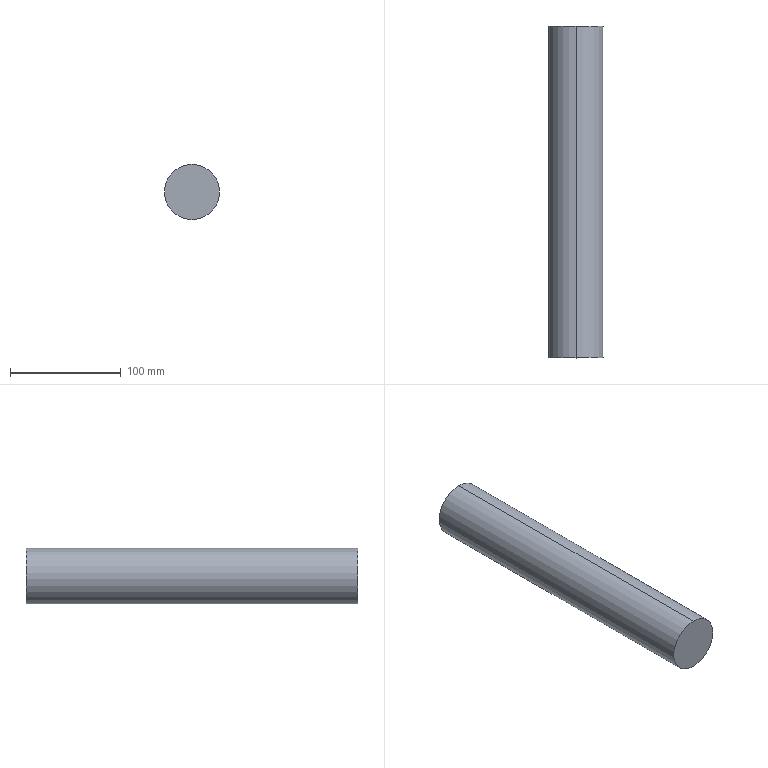Part | STEP file | Tie rod 2 | 1 solid | 4 faces | box 50 x 300 x 50 mm | volume 589049 mm3 | cylinder 2 | plane 2 | commonest cylinder face diameters 50 x2
STEP:
#1=CARTESIAN_POINT('',(0.,300.,25.));
#2=VERTEX_POINT('',#1);
#3=CARTESIAN_POINT('',(0.,300.,-25.));
#4=VERTEX_POINT('',#3);
#5=CARTESIAN_POINT('',(0.,300.,0.));
#6=DIRECTION('',(0.,1.,0.));
#7=DIRECTION('',(0.,0.,1.));
#8=AXIS2_PLACEMENT_3D('',#5,#6,#7);
#9=CIRCLE('',#8,25.);
#10=EDGE_CURVE('',#2,#4,#9,.T.);
#11=ORIENTED_EDGE('',*,*,#10,.F.);
#12=CARTESIAN_POINT('',(0.,0.,25.));
#13=VERTEX_POINT('',#12);
#14=CARTESIAN_POINT('',(0.,300.,25.));
#15=DIRECTION('',(0.,-1.,0.));
#16=VECTOR('',#15,1000.);
#17=LINE('',#14,#16);
#18=EDGE_CURVE('',#2,#13,#17,.T.);
#19=ORIENTED_EDGE('',*,*,#18,.T.);
#20=CARTESIAN_POINT('',(0.,0.,-25.));
#21=VERTEX_POINT('',#20);
#22=CARTESIAN_POINT('',(0.,0.,0.));
#23=DIRECTION('',(0.,1.,0.));
#24=DIRECTION('',(0.,0.,1.));
#25=AXIS2_PLACEMENT_3D('',#22,#23,#24);
#26=CIRCLE('',#25,25.);
#27=EDGE_CURVE('',#13,#21,#26,.T.);
#28=ORIENTED_EDGE('',*,*,#27,.T.);
#29=CARTESIAN_POINT('',(0.,300.,-25.));
#30=DIRECTION('',(0.,-1.,0.));
#31=VECTOR('',#30,1000.);
#32=LINE('',#29,#31);
#33=EDGE_CURVE('',#4,#21,#32,.T.);
#34=ORIENTED_EDGE('',*,*,#33,.F.);
#35=EDGE_LOOP('',(#11,#19,#28,#34));
#36=FACE_OUTER_BOUND('',#35,.T.);
#37=CARTESIAN_POINT('',(0.,300.,0.));
#38=DIRECTION('',(0.,-1.,0.));
#39=DIRECTION('',(0.,0.,-1.));
#40=AXIS2_PLACEMENT_3D('',#37,#38,#39);
#41=CYLINDRICAL_SURFACE('',#40,25.);
#42=ADVANCED_FACE('',(#36),#41,.T.);
#43=ORIENTED_EDGE('',*,*,#18,.F.);
#44=CARTESIAN_POINT('',(0.,300.,0.));
#45=DIRECTION('',(0.,1.,0.));
#46=DIRECTION('',(0.,0.,1.));
#47=AXIS2_PLACEMENT_3D('',#44,#45,#46);
#48=CIRCLE('',#47,25.);
#49=EDGE_CURVE('',#4,#2,#48,.T.);
#50=ORIENTED_EDGE('',*,*,#49,.F.);
#51=ORIENTED_EDGE('',*,*,#33,.T.);
#52=CARTESIAN_POINT('',(0.,0.,0.));
#53=DIRECTION('',(0.,1.,0.));
#54=DIRECTION('',(0.,0.,1.));
#55=AXIS2_PLACEMENT_3D('',#52,#53,#54);
#56=CIRCLE('',#55,25.);
#57=EDGE_CURVE('',#21,#13,#56,.T.);
#58=ORIENTED_EDGE('',*,*,#57,.T.);
#59=EDGE_LOOP('',(#43,#50,#51,#58));
#60=FACE_OUTER_BOUND('',#59,.T.);
#61=CARTESIAN_POINT('',(0.,300.,0.));
#62=DIRECTION('',(0.,-1.,0.));
#63=DIRECTION('',(0.,0.,-1.));
#64=AXIS2_PLACEMENT_3D('',#61,#62,#63);
#65=CYLINDRICAL_SURFACE('',#64,25.);
#66=ADVANCED_FACE('',(#60),#65,.T.);
#67=ORIENTED_EDGE('',*,*,#49,.T.);
#68=ORIENTED_EDGE('',*,*,#10,.T.);
#69=EDGE_LOOP('',(#67,#68));
#70=FACE_OUTER_BOUND('',#69,.T.);
#71=CARTESIAN_POINT('',(0.,300.,0.));
#72=DIRECTION('',(0.,1.,0.));
#73=DIRECTION('',(0.,0.,1.));
#74=AXIS2_PLACEMENT_3D('',#71,#72,#73);
#75=PLANE('',#74);
#76=ADVANCED_FACE('',(#70),#75,.T.);
#77=ORIENTED_EDGE('',*,*,#57,.F.);
#78=ORIENTED_EDGE('',*,*,#27,.F.);
#79=EDGE_LOOP('',(#77,#78));
#80=FACE_OUTER_BOUND('',#79,.T.);
#81=CARTESIAN_POINT('',(0.,0.,0.));
#82=DIRECTION('',(0.,1.,0.));
#83=DIRECTION('',(0.,0.,1.));
#84=AXIS2_PLACEMENT_3D('',#81,#82,#83);
#85=PLANE('',#84);
#86=ADVANCED_FACE('',(#80),#85,.F.);
#87=CLOSED_SHELL('',(#42,#66,#76,#86));
#88=MANIFOLD_SOLID_BREP('',#87);
#89=CARTESIAN_POINT('',(0.,0.,0.));
#90=DIRECTION('',(0.,0.,1.));
#91=DIRECTION('',(1.,0.,0.));
#92=AXIS2_PLACEMENT_3D('',#89,#90,#91);
#93=(LENGTH_UNIT()NAMED_UNIT(*)SI_UNIT(.MILLI.,.METRE.));
#94=UNCERTAINTY_MEASURE_WITH_UNIT(LENGTH_MEASURE(0.00001),#93,'','');
#95=(NAMED_UNIT(*)PLANE_ANGLE_UNIT()SI_UNIT($,.RADIAN.));
#96=(NAMED_UNIT(*)SI_UNIT($,.STERADIAN.)SOLID_ANGLE_UNIT());
#97=(GEOMETRIC_REPRESENTATION_CONTEXT(3)GLOBAL_UNCERTAINTY_ASSIGNED_CONTEXT((#94))GLOBAL_UNIT_ASSIGNED_CONTEXT((#93,#95,#96))REPRESENTATION_CONTEXT('',''));
#98=ADVANCED_BREP_SHAPE_REPRESENTATION('',(#88,#92),#97);